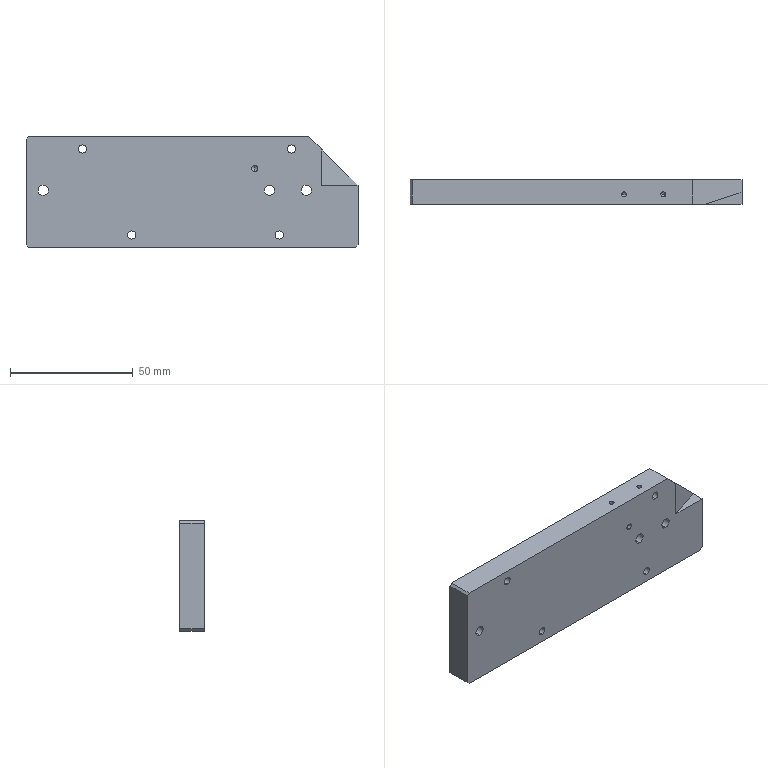Part | SolidWorks | features ICE 14, HoleWzd 6, Chamfer 3, 3DProfileFeature 2, Extrusion 1, Fillet 1, LPattern 1 | 1 solid | 67 faces | box 135 x 10 x 45 mm | volume 55764 mm3 | cylinder 34 | plane 21 | cone 12 | commonest cylinder face diameters 4.2 x12 3.3 x8 5 x8 2.05 x4 2.5 x2